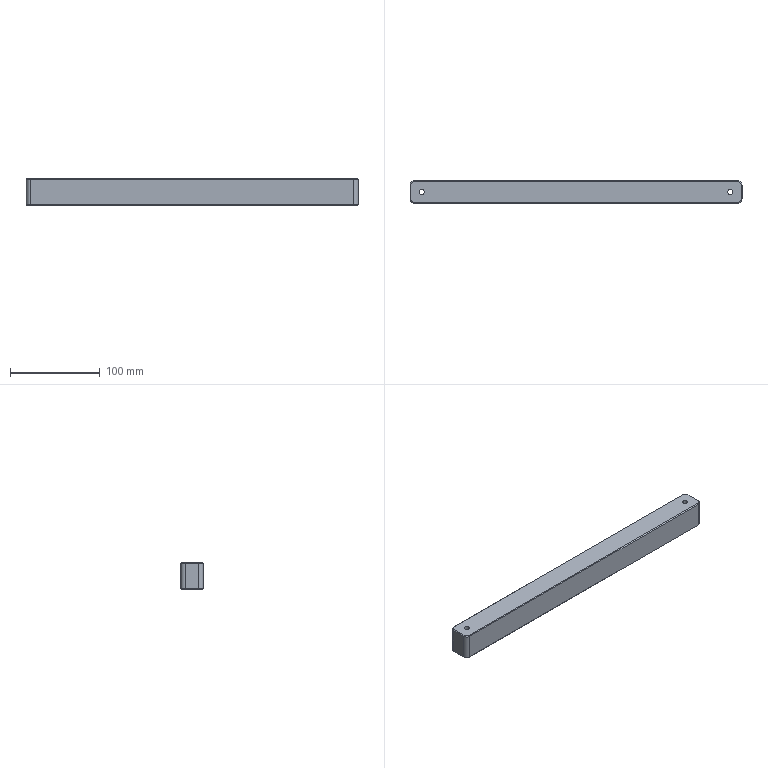Part | SolidWorks | features Chamfer 1, Extrusion 1, Fillet 1, HoleWzd 1 | 1 solid | 36 faces | box 370 x 25 x 30 mm | volume 274027 mm3 | plane 16 | cylinder 12 | cone 8 | commonest cylinder face diameters 10 x8 5.5 x4
STEP:
#1=CARTESIAN_POINT('',(177.,0.,-9.3));
#2=VERTEX_POINT('',#1);
#3=CARTESIAN_POINT('',(167.,0.,-9.3));
#4=VERTEX_POINT('',#3);
#5=CARTESIAN_POINT('',(172.,0.,-9.3));
#6=DIRECTION('',(0.,0.,-1.));
#7=DIRECTION('',(-1.,0.,0.));
#8=AXIS2_PLACEMENT_3D('',#5,#6,#7);
#9=CIRCLE('',#8,5.);
#10=EDGE_CURVE('',#2,#4,#9,.T.);
#11=ORIENTED_EDGE('',*,*,#10,.F.);
#12=CARTESIAN_POINT('',(177.,0.,-15.));
#13=VERTEX_POINT('',#12);
#14=CARTESIAN_POINT('',(177.,0.,-15.));
#15=DIRECTION('',(0.,0.,-1.));
#16=VECTOR('',#15,1000.);
#17=LINE('',#14,#16);
#18=EDGE_CURVE('',#2,#13,#17,.T.);
#19=ORIENTED_EDGE('',*,*,#18,.T.);
#20=CARTESIAN_POINT('',(167.,0.,-15.));
#21=VERTEX_POINT('',#20);
#22=CARTESIAN_POINT('',(172.,0.,-15.));
#23=DIRECTION('',(0.,0.,-1.));
#24=DIRECTION('',(-1.,0.,0.));
#25=AXIS2_PLACEMENT_3D('',#22,#23,#24);
#26=CIRCLE('',#25,5.);
#27=EDGE_CURVE('',#13,#21,#26,.T.);
#28=ORIENTED_EDGE('',*,*,#27,.T.);
#29=CARTESIAN_POINT('',(167.,0.,-15.));
#30=DIRECTION('',(0.,0.,-1.));
#31=VECTOR('',#30,1000.);
#32=LINE('',#29,#31);
#33=EDGE_CURVE('',#4,#21,#32,.T.);
#34=ORIENTED_EDGE('',*,*,#33,.F.);
#35=EDGE_LOOP('',(#11,#19,#28,#34));
#36=FACE_OUTER_BOUND('',#35,.T.);
#37=CARTESIAN_POINT('',(172.,0.,-15.));
#38=DIRECTION('',(0.,0.,-1.));
#39=DIRECTION('',(-1.,0.,0.));
#40=AXIS2_PLACEMENT_3D('',#37,#38,#39);
#41=CYLINDRICAL_SURFACE('',#40,5.);
#42=ADVANCED_FACE('',(#36),#41,.F.);
#43=CARTESIAN_POINT('',(174.75,0.,15.));
#44=VERTEX_POINT('',#43);
#45=CARTESIAN_POINT('',(169.25,0.,15.));
#46=VERTEX_POINT('',#45);
#47=CARTESIAN_POINT('',(172.,0.,15.));
#48=DIRECTION('',(0.,0.,-1.));
#49=DIRECTION('',(-1.,0.,0.));
#50=AXIS2_PLACEMENT_3D('',#47,#48,#49);
#51=CIRCLE('',#50,2.75);
#52=EDGE_CURVE('',#44,#46,#51,.T.);
#53=ORIENTED_EDGE('',*,*,#52,.F.);
#54=CARTESIAN_POINT('',(174.75,0.,-9.3));
#55=VERTEX_POINT('',#54);
#56=CARTESIAN_POINT('',(174.75,0.,-15.));
#57=DIRECTION('',(0.,0.,-1.));
#58=VECTOR('',#57,1000.);
#59=LINE('',#56,#58);
#60=EDGE_CURVE('',#44,#55,#59,.T.);
#61=ORIENTED_EDGE('',*,*,#60,.T.);
#62=CARTESIAN_POINT('',(169.25,0.,-9.3));
#63=VERTEX_POINT('',#62);
#64=CARTESIAN_POINT('',(172.,0.,-9.3));
#65=DIRECTION('',(0.,0.,-1.));
#66=DIRECTION('',(-1.,0.,0.));
#67=AXIS2_PLACEMENT_3D('',#64,#65,#66);
#68=CIRCLE('',#67,2.75);
#69=EDGE_CURVE('',#55,#63,#68,.T.);
#70=ORIENTED_EDGE('',*,*,#69,.T.);
#71=CARTESIAN_POINT('',(169.25,0.,-15.));
#72=DIRECTION('',(0.,0.,-1.));
#73=VECTOR('',#72,1000.);
#74=LINE('',#71,#73);
#75=EDGE_CURVE('',#46,#63,#74,.T.);
#76=ORIENTED_EDGE('',*,*,#75,.F.);
#77=EDGE_LOOP('',(#53,#61,#70,#76));
#78=FACE_OUTER_BOUND('',#77,.T.);
#79=CARTESIAN_POINT('',(172.,0.,-15.));
#80=DIRECTION('',(0.,0.,-1.));
#81=DIRECTION('',(-1.,0.,0.));
#82=AXIS2_PLACEMENT_3D('',#79,#80,#81);
#83=CYLINDRICAL_SURFACE('',#82,2.75);
#84=ADVANCED_FACE('',(#78),#83,.F.);
#85=CARTESIAN_POINT('',(-167.,0.,-9.3));
#86=VERTEX_POINT('',#85);
#87=CARTESIAN_POINT('',(-177.,0.,-9.3));
#88=VERTEX_POINT('',#87);
#89=CARTESIAN_POINT('',(-172.,0.,-9.3));
#90=DIRECTION('',(0.,0.,-1.));
#91=DIRECTION('',(-1.,0.,0.));
#92=AXIS2_PLACEMENT_3D('',#89,#90,#91);
#93=CIRCLE('',#92,5.);
#94=EDGE_CURVE('',#86,#88,#93,.T.);
#95=ORIENTED_EDGE('',*,*,#94,.F.);
#96=CARTESIAN_POINT('',(-167.,0.,-15.));
#97=VERTEX_POINT('',#96);
#98=CARTESIAN_POINT('',(-167.,0.,-15.));
#99=DIRECTION('',(0.,0.,-1.));
#100=VECTOR('',#99,1000.);
#101=LINE('',#98,#100);
#102=EDGE_CURVE('',#86,#97,#101,.T.);
#103=ORIENTED_EDGE('',*,*,#102,.T.);
#104=CARTESIAN_POINT('',(-177.,0.,-15.));
#105=VERTEX_POINT('',#104);
#106=CARTESIAN_POINT('',(-172.,0.,-15.));
#107=DIRECTION('',(0.,0.,-1.));
#108=DIRECTION('',(-1.,0.,0.));
#109=AXIS2_PLACEMENT_3D('',#106,#107,#108);
#110=CIRCLE('',#109,5.);
#111=EDGE_CURVE('',#97,#105,#110,.T.);
#112=ORIENTED_EDGE('',*,*,#111,.T.);
#113=CARTESIAN_POINT('',(-177.,0.,-15.));
#114=DIRECTION('',(0.,0.,-1.));
#115=VECTOR('',#114,1000.);
#116=LINE('',#113,#115);
#117=EDGE_CURVE('',#88,#105,#116,.T.);
#118=ORIENTED_EDGE('',*,*,#117,.F.);
#119=EDGE_LOOP('',(#95,#103,#112,#118));
#120=FACE_OUTER_BOUND('',#119,.T.);
#121=CARTESIAN_POINT('',(-172.,0.,-15.));
#122=DIRECTION('',(0.,0.,-1.));
#123=DIRECTION('',(-1.,0.,0.));
#124=AXIS2_PLACEMENT_3D('',#121,#122,#123);
#125=CYLINDRICAL_SURFACE('',#124,5.);
#126=ADVANCED_FACE('',(#120),#125,.F.);
#127=CARTESIAN_POINT('',(-169.25,0.,15.));
#128=VERTEX_POINT('',#127);
#129=CARTESIAN_POINT('',(-174.75,0.,15.));
#130=VERTEX_POINT('',#129);
#131=CARTESIAN_POINT('',(-172.,0.,15.));
#132=DIRECTION('',(0.,0.,-1.));
#133=DIRECTION('',(-1.,0.,0.));
#134=AXIS2_PLACEMENT_3D('',#131,#132,#133);
#135=CIRCLE('',#134,2.75);
#136=EDGE_CURVE('',#128,#130,#135,.T.);
#137=ORIENTED_EDGE('',*,*,#136,.F.);
#138=CARTESIAN_POINT('',(-169.25,0.,-9.3));
#139=VERTEX_POINT('',#138);
#140=CARTESIAN_POINT('',(-169.25,0.,-15.));
#141=DIRECTION('',(0.,0.,-1.));
#142=VECTOR('',#141,1000.);
#143=LINE('',#140,#142);
#144=EDGE_CURVE('',#128,#139,#143,.T.);
#145=ORIENTED_EDGE('',*,*,#144,.T.);
#146=CARTESIAN_POINT('',(-174.75,0.,-9.3));
#147=VERTEX_POINT('',#146);
#148=CARTESIAN_POINT('',(-172.,0.,-9.3));
#149=DIRECTION('',(0.,0.,-1.));
#150=DIRECTION('',(-1.,0.,0.));
#151=AXIS2_PLACEMENT_3D('',#148,#149,#150);
#152=CIRCLE('',#151,2.75);
#153=EDGE_CURVE('',#139,#147,#152,.T.);
#154=ORIENTED_EDGE('',*,*,#153,.T.);
#155=CARTESIAN_POINT('',(-174.75,0.,-15.));
#156=DIRECTION('',(0.,0.,-1.));
#157=VECTOR('',#156,1000.);
#158=LINE('',#155,#157);
#159=EDGE_CURVE('',#130,#147,#158,.T.);
#160=ORIENTED_EDGE('',*,*,#159,.F.);
#161=EDGE_LOOP('',(#137,#145,#154,#160));
#162=FACE_OUTER_BOUND('',#161,.T.);
#163=CARTESIAN_POINT('',(-172.,0.,-15.));
#164=DIRECTION('',(0.,0.,-1.));
#165=DIRECTION('',(-1.,0.,0.));
#166=AXIS2_PLACEMENT_3D('',#163,#164,#165);
#167=CYLINDRICAL_SURFACE('',#166,2.75);
#168=ADVANCED_FACE('',(#162),#167,.F.);
#169=CARTESIAN_POINT('',(185.,7.5,-14.));
#170=VERTEX_POINT('',#169);
#171=CARTESIAN_POINT('',(185.,7.5,14.));
#172=VERTEX_POINT('',#171);
#173=CARTESIAN_POINT('',(185.,7.5,15.));
#174=DIRECTION('',(0.,0.,1.));
#175=VECTOR('',#174,1000.);
#176=LINE('',#173,#175);
#177=EDGE_CURVE('',#170,#172,#176,.T.);
#178=ORIENTED_EDGE('',*,*,#177,.T.);
#179=CARTESIAN_POINT('',(185.,-7.5,14.));
#180=VERTEX_POINT('',#179);
#181=CARTESIAN_POINT('',(185.,-7.5,14.));
#182=DIRECTION('',(0.,-1.,0.));
#183=VECTOR('',#182,1000.);
#184=LINE('',#181,#183);
#185=EDGE_CURVE('',#172,#180,#184,.T.);
#186=ORIENTED_EDGE('',*,*,#185,.T.);
#187=CARTESIAN_POINT('',(185.,-7.5,-14.));
#188=VERTEX_POINT('',#187);
#189=CARTESIAN_POINT('',(185.,-7.5,15.));
#190=DIRECTION('',(0.,0.,-1.));
#191=VECTOR('',#190,1000.);
#192=LINE('',#189,#191);
#193=EDGE_CURVE('',#180,#188,#192,.T.);
#194=ORIENTED_EDGE('',*,*,#193,.T.);
#195=CARTESIAN_POINT('',(185.,12.5,-14.));
#196=DIRECTION('',(0.,1.,0.));
#197=VECTOR('',#196,1000.);
#198=LINE('',#195,#197);
#199=EDGE_CURVE('',#188,#170,#198,.T.);
#200=ORIENTED_EDGE('',*,*,#199,.T.);
#201=EDGE_LOOP('',(#178,#186,#194,#200));
#202=FACE_OUTER_BOUND('',#201,.T.);
#203=CARTESIAN_POINT('',(185.,12.5,15.));
#204=DIRECTION('',(-1.,0.,0.));
#205=DIRECTION('',(0.,0.,1.));
#206=AXIS2_PLACEMENT_3D('',#203,#204,#205);
#207=PLANE('',#206);
#208=ADVANCED_FACE('',(#202),#207,.F.);
#209=CARTESIAN_POINT('',(-180.,12.5,-14.));
#210=VERTEX_POINT('',#209);
#211=CARTESIAN_POINT('',(-180.,12.5,14.));
#212=VERTEX_POINT('',#211);
#213=CARTESIAN_POINT('',(-180.,12.5,15.));
#214=DIRECTION('',(0.,0.,1.));
#215=VECTOR('',#214,1000.);
#216=LINE('',#213,#215);
#217=EDGE_CURVE('',#210,#212,#216,.T.);
#218=ORIENTED_EDGE('',*,*,#217,.T.);
#219=CARTESIAN_POINT('',(180.,12.5,14.));
#220=VERTEX_POINT('',#219);
#221=CARTESIAN_POINT('',(180.,12.5,14.));
#222=DIRECTION('',(1.,0.,0.));
#223=VECTOR('',#222,1000.);
#224=LINE('',#221,#223);
#225=EDGE_CURVE('',#212,#220,#224,.T.);
#226=ORIENTED_EDGE('',*,*,#225,.T.);
#227=CARTESIAN_POINT('',(180.,12.5,-14.));
#228=VERTEX_POINT('',#227);
#229=CARTESIAN_POINT('',(180.,12.5,15.));
#230=DIRECTION('',(0.,0.,-1.));
#231=VECTOR('',#230,1000.);
#232=LINE('',#229,#231);
#233=EDGE_CURVE('',#220,#228,#232,.T.);
#234=ORIENTED_EDGE('',*,*,#233,.T.);
#235=CARTESIAN_POINT('',(-185.,12.5,-14.));
#236=DIRECTION('',(-1.,0.,0.));
#237=VECTOR('',#236,1000.);
#238=LINE('',#235,#237);
#239=EDGE_CURVE('',#228,#210,#238,.T.);
#240=ORIENTED_EDGE('',*,*,#239,.T.);
#241=EDGE_LOOP('',(#218,#226,#234,#240));
#242=FACE_OUTER_BOUND('',#241,.T.);
#243=CARTESIAN_POINT('',(-185.,12.5,15.));
#244=DIRECTION('',(0.,-1.,0.));
#245=DIRECTION('',(0.,0.,-1.));
#246=AXIS2_PLACEMENT_3D('',#243,#244,#245);
#247=PLANE('',#246);
#248=ADVANCED_FACE('',(#242),#247,.F.);
#249=CARTESIAN_POINT('',(-185.,-7.5,-14.));
#250=VERTEX_POINT('',#249);
#251=CARTESIAN_POINT('',(-185.,-7.5,14.));
#252=VERTEX_POINT('',#251);
#253=CARTESIAN_POINT('',(-185.,-7.5,15.));
#254=DIRECTION('',(0.,0.,1.));
#255=VECTOR('',#254,1000.);
#256=LINE('',#253,#255);
#257=EDGE_CURVE('',#250,#252,#256,.T.);
#258=ORIENTED_EDGE('',*,*,#257,.T.);
#259=CARTESIAN_POINT('',(-185.,7.5,14.));
#260=VERTEX_POINT('',#259);
#261=CARTESIAN_POINT('',(-185.,7.5,14.));
#262=DIRECTION('',(0.,1.,0.));
#263=VECTOR('',#262,1000.);
#264=LINE('',#261,#263);
#265=EDGE_CURVE('',#252,#260,#264,.T.);
#266=ORIENTED_EDGE('',*,*,#265,.T.);
#267=CARTESIAN_POINT('',(-185.,7.5,-14.));
#268=VERTEX_POINT('',#267);
#269=CARTESIAN_POINT('',(-185.,7.5,15.));
#270=DIRECTION('',(0.,0.,-1.));
#271=VECTOR('',#270,1000.);
#272=LINE('',#269,#271);
#273=EDGE_CURVE('',#260,#268,#272,.T.);
#274=ORIENTED_EDGE('',*,*,#273,.T.);
#275=CARTESIAN_POINT('',(-185.,12.5,-14.));
#276=DIRECTION('',(0.,-1.,0.));
#277=VECTOR('',#276,1000.);
#278=LINE('',#275,#277);
#279=EDGE_CURVE('',#268,#250,#278,.T.);
#280=ORIENTED_EDGE('',*,*,#279,.T.);
#281=EDGE_LOOP('',(#258,#266,#274,#280));
#282=FACE_OUTER_BOUND('',#281,.T.);
#283=CARTESIAN_POINT('',(-185.,12.5,15.));
#284=DIRECTION('',(1.,0.,0.));
#285=DIRECTION('',(0.,0.,-1.));
#286=AXIS2_PLACEMENT_3D('',#283,#284,#285);
#287=PLANE('',#286);
#288=ADVANCED_FACE('',(#282),#287,.F.);
#289=CARTESIAN_POINT('',(180.,-12.5,-14.));
#290=VERTEX_POINT('',#289);
#291=CARTESIAN_POINT('',(180.,-12.5,14.));
#292=VERTEX_POINT('',#291);
#293=CARTESIAN_POINT('',(180.,-12.5,15.));
#294=DIRECTION('',(0.,0.,1.));
#295=VECTOR('',#294,1000.);
#296=LINE('',#293,#295);
#297=EDGE_CURVE('',#290,#292,#296,.T.);
#298=ORIENTED_EDGE('',*,*,#297,.T.);
#299=CARTESIAN_POINT('',(-180.,-12.5,14.));
#300=VERTEX_POINT('',#299);
#301=CARTESIAN_POINT('',(-180.,-12.5,14.));
#302=DIRECTION('',(-1.,0.,0.));
#303=VECTOR('',#302,1000.);
#304=LINE('',#301,#303);
#305=EDGE_CURVE('',#292,#300,#304,.T.);
#306=ORIENTED_EDGE('',*,*,#305,.T.);
#307=CARTESIAN_POINT('',(-180.,-12.5,-14.));
#308=VERTEX_POINT('',#307);
#309=CARTESIAN_POINT('',(-180.,-12.5,15.));
#310=DIRECTION('',(0.,0.,-1.));
#311=VECTOR('',#310,1000.);
#312=LINE('',#309,#311);
#313=EDGE_CURVE('',#300,#308,#312,.T.);
#314=ORIENTED_EDGE('',*,*,#313,.T.);
#315=CARTESIAN_POINT('',(-185.,-12.5,-14.));
#316=DIRECTION('',(1.,0.,0.));
#317=VECTOR('',#316,1000.);
#318=LINE('',#315,#317);
#319=EDGE_CURVE('',#308,#290,#318,.T.);
#320=ORIENTED_EDGE('',*,*,#319,.T.);
#321=EDGE_LOOP('',(#298,#306,#314,#320));
#322=FACE_OUTER_BOUND('',#321,.T.);
#323=CARTESIAN_POINT('',(-185.,-12.5,15.));
#324=DIRECTION('',(0.,1.,0.));
#325=DIRECTION('',(0.,0.,1.));
#326=AXIS2_PLACEMENT_3D('',#323,#324,#325);
#327=PLANE('',#326);
#328=ADVANCED_FACE('',(#322),#327,.F.);
#329=CARTESIAN_POINT('',(172.,0.,15.));
#330=DIRECTION('',(0.,0.,-1.));
#331=DIRECTION('',(-1.,0.,0.));
#332=AXIS2_PLACEMENT_3D('',#329,#330,#331);
#333=CIRCLE('',#332,2.75);
#334=EDGE_CURVE('',#46,#44,#333,.T.);
#335=ORIENTED_EDGE('',*,*,#334,.T.);
#336=ORIENTED_EDGE('',*,*,#52,.T.);
#337=EDGE_LOOP('',(#335,#336));
#338=FACE_BOUND('',#337,.T.);
#339=CARTESIAN_POINT('',(-172.,0.,15.));
#340=DIRECTION('',(0.,0.,-1.));
#341=DIRECTION('',(-1.,0.,0.));
#342=AXIS2_PLACEMENT_3D('',#339,#340,#341);
#343=CIRCLE('',#342,2.75);
#344=EDGE_CURVE('',#130,#128,#343,.T.);
#345=ORIENTED_EDGE('',*,*,#344,.T.);
#346=ORIENTED_EDGE('',*,*,#136,.T.);
#347=EDGE_LOOP('',(#345,#346));
#348=FACE_BOUND('',#347,.T.);
#349=CARTESIAN_POINT('',(184.,-7.5,15.));
#350=VERTEX_POINT('',#349);
#351=CARTESIAN_POINT('',(184.,7.5,15.));
#352=VERTEX_POINT('',#351);
#353=CARTESIAN_POINT('',(184.,7.5,15.));
#354=DIRECTION('',(0.,1.,0.));
#355=VECTOR('',#354,1000.);
#356=LINE('',#353,#355);
#357=EDGE_CURVE('',#350,#352,#356,.T.);
#358=ORIENTED_EDGE('',*,*,#357,.T.);
#359=CARTESIAN_POINT('',(180.,11.5,15.));
#360=VERTEX_POINT('',#359);
#361=CARTESIAN_POINT('',(180.,7.5,15.));
#362=DIRECTION('',(0.,0.,1.));
#363=DIRECTION('',(1.,0.,0.));
#364=AXIS2_PLACEMENT_3D('',#361,#362,#363);
#365=CIRCLE('',#364,4.);
#366=EDGE_CURVE('',#352,#360,#365,.T.);
#367=ORIENTED_EDGE('',*,*,#366,.T.);
#368=CARTESIAN_POINT('',(-180.,11.5,15.));
#369=VERTEX_POINT('',#368);
#370=CARTESIAN_POINT('',(-180.,11.5,15.));
#371=DIRECTION('',(-1.,0.,0.));
#372=VECTOR('',#371,1000.);
#373=LINE('',#370,#372);
#374=EDGE_CURVE('',#360,#369,#373,.T.);
#375=ORIENTED_EDGE('',*,*,#374,.T.);
#376=CARTESIAN_POINT('',(-184.,7.5,15.));
#377=VERTEX_POINT('',#376);
#378=CARTESIAN_POINT('',(-180.,7.5,15.));
#379=DIRECTION('',(0.,0.,1.));
#380=DIRECTION('',(1.,0.,0.));
#381=AXIS2_PLACEMENT_3D('',#378,#379,#380);
#382=CIRCLE('',#381,4.);
#383=EDGE_CURVE('',#369,#377,#382,.T.);
#384=ORIENTED_EDGE('',*,*,#383,.T.);
#385=CARTESIAN_POINT('',(-184.,-7.5,15.));
#386=VERTEX_POINT('',#385);
#387=CARTESIAN_POINT('',(-184.,-7.5,15.));
#388=DIRECTION('',(0.,-1.,0.));
#389=VECTOR('',#388,1000.);
#390=LINE('',#387,#389);
#391=EDGE_CURVE('',#377,#386,#390,.T.);
#392=ORIENTED_EDGE('',*,*,#391,.T.);
#393=CARTESIAN_POINT('',(-180.,-11.5,15.));
#394=VERTEX_POINT('',#393);
#395=CARTESIAN_POINT('',(-180.,-7.5,15.));
#396=DIRECTION('',(0.,0.,1.));
#397=DIRECTION('',(1.,0.,0.));
#398=AXIS2_PLACEMENT_3D('',#395,#396,#397);
#399=CIRCLE('',#398,4.);
#400=EDGE_CURVE('',#386,#394,#399,.T.);
#401=ORIENTED_EDGE('',*,*,#400,.T.);
#402=CARTESIAN_POINT('',(180.,-11.5,15.));
#403=VERTEX_POINT('',#402);
#404=CARTESIAN_POINT('',(180.,-11.5,15.));
#405=DIRECTION('',(1.,0.,0.));
#406=VECTOR('',#405,1000.);
#407=LINE('',#404,#406);
#408=EDGE_CURVE('',#394,#403,#407,.T.);
#409=ORIENTED_EDGE('',*,*,#408,.T.);
#410=CARTESIAN_POINT('',(180.,-7.5,15.));
#411=DIRECTION('',(0.,0.,1.));
#412=DIRECTION('',(1.,0.,0.));
#413=AXIS2_PLACEMENT_3D('',#410,#411,#412);
#414=CIRCLE('',#413,4.);
#415=EDGE_CURVE('',#403,#350,#414,.T.);
#416=ORIENTED_EDGE('',*,*,#415,.T.);
#417=EDGE_LOOP('',(#358,#367,#375,#384,#392,#401,#409,#416));
#418=FACE_OUTER_BOUND('',#417,.T.);
#419=CARTESIAN_POINT('',(185.,-12.5,15.));
#420=DIRECTION('',(0.,0.,1.));
#421=DIRECTION('',(1.,0.,0.));
#422=AXIS2_PLACEMENT_3D('',#419,#420,#421);
#423=PLANE('',#422);
#424=ADVANCED_FACE('',(#338,#348,#418),#423,.T.);
#425=CARTESIAN_POINT('',(172.,0.,-15.));
#426=DIRECTION('',(0.,0.,-1.));
#427=DIRECTION('',(-1.,0.,0.));
#428=AXIS2_PLACEMENT_3D('',#425,#426,#427);
#429=CIRCLE('',#428,5.);
#430=EDGE_CURVE('',#21,#13,#429,.T.);
#431=ORIENTED_EDGE('',*,*,#430,.F.);
#432=ORIENTED_EDGE('',*,*,#27,.F.);
#433=EDGE_LOOP('',(#431,#432));
#434=FACE_BOUND('',#433,.T.);
#435=CARTESIAN_POINT('',(-172.,0.,-15.));
#436=DIRECTION('',(0.,0.,-1.));
#437=DIRECTION('',(-1.,0.,0.));
#438=AXIS2_PLACEMENT_3D('',#435,#436,#437);
#439=CIRCLE('',#438,5.);
#440=EDGE_CURVE('',#105,#97,#439,.T.);
#441=ORIENTED_EDGE('',*,*,#440,.F.);
#442=ORIENTED_EDGE('',*,*,#111,.F.);
#443=EDGE_LOOP('',(#441,#442));
#444=FACE_BOUND('',#443,.T.);
#445=CARTESIAN_POINT('',(-184.,7.5,-15.));
#446=VERTEX_POINT('',#445);
#447=CARTESIAN_POINT('',(-180.,11.5,-15.));
#448=VERTEX_POINT('',#447);
#449=CARTESIAN_POINT('',(-180.,7.5,-15.));
#450=DIRECTION('',(0.,0.,-1.));
#451=DIRECTION('',(1.,0.,0.));
#452=AXIS2_PLACEMENT_3D('',#449,#450,#451);
#453=CIRCLE('',#452,4.);
#454=EDGE_CURVE('',#446,#448,#453,.T.);
#455=ORIENTED_EDGE('',*,*,#454,.T.);
#456=CARTESIAN_POINT('',(180.,11.5,-15.));
#457=VERTEX_POINT('',#456);
#458=CARTESIAN_POINT('',(185.,11.5,-15.));
#459=DIRECTION('',(1.,0.,0.));
#460=VECTOR('',#459,1000.);
#461=LINE('',#458,#460);
#462=EDGE_CURVE('',#448,#457,#461,.T.);
#463=ORIENTED_EDGE('',*,*,#462,.T.);
#464=CARTESIAN_POINT('',(184.,7.5,-15.));
#465=VERTEX_POINT('',#464);
#466=CARTESIAN_POINT('',(180.,7.5,-15.));
#467=DIRECTION('',(0.,0.,-1.));
#468=DIRECTION('',(1.,0.,0.));
#469=AXIS2_PLACEMENT_3D('',#466,#467,#468);
#470=CIRCLE('',#469,4.);
#471=EDGE_CURVE('',#457,#465,#470,.T.);
#472=ORIENTED_EDGE('',*,*,#471,.T.);
#473=CARTESIAN_POINT('',(184.,-7.5,-15.));
#474=VERTEX_POINT('',#473);
#475=CARTESIAN_POINT('',(184.,-12.5,-15.));
#476=DIRECTION('',(0.,-1.,0.));
#477=VECTOR('',#476,1000.);
#478=LINE('',#475,#477);
#479=EDGE_CURVE('',#465,#474,#478,.T.);
#480=ORIENTED_EDGE('',*,*,#479,.T.);
#481=CARTESIAN_POINT('',(180.,-11.5,-15.));
#482=VERTEX_POINT('',#481);
#483=CARTESIAN_POINT('',(180.,-7.5,-15.));
#484=DIRECTION('',(0.,0.,-1.));
#485=DIRECTION('',(1.,0.,0.));
#486=AXIS2_PLACEMENT_3D('',#483,#484,#485);
#487=CIRCLE('',#486,4.);
#488=EDGE_CURVE('',#474,#482,#487,.T.);
#489=ORIENTED_EDGE('',*,*,#488,.T.);
#490=CARTESIAN_POINT('',(-180.,-11.5,-15.));
#491=VERTEX_POINT('',#490);
#492=CARTESIAN_POINT('',(185.,-11.5,-15.));
#493=DIRECTION('',(-1.,0.,0.));
#494=VECTOR('',#493,1000.);
#495=LINE('',#492,#494);
#496=EDGE_CURVE('',#482,#491,#495,.T.);
#497=ORIENTED_EDGE('',*,*,#496,.T.);
#498=CARTESIAN_POINT('',(-184.,-7.5,-15.));
#499=VERTEX_POINT('',#498);
#500=CARTESIAN_POINT('',(-180.,-7.5,-15.));
#501=DIRECTION('',(0.,0.,-1.));
#502=DIRECTION('',(1.,0.,0.));
#503=AXIS2_PLACEMENT_3D('',#500,#501,#502);
#504=CIRCLE('',#503,4.);
#505=EDGE_CURVE('',#491,#499,#504,.T.);
#506=ORIENTED_EDGE('',*,*,#505,.T.);
#507=CARTESIAN_POINT('',(-184.,-12.5,-15.));
#508=DIRECTION('',(0.,1.,0.));
#509=VECTOR('',#508,1000.);
#510=LINE('',#507,#509);
#511=EDGE_CURVE('',#499,#446,#510,.T.);
#512=ORIENTED_EDGE('',*,*,#511,.T.);
#513=EDGE_LOOP('',(#455,#463,#472,#480,#489,#497,#506,#512));
#514=FACE_OUTER_BOUND('',#513,.T.);
#515=CARTESIAN_POINT('',(185.,-12.5,-15.));
#516=DIRECTION('',(0.,0.,1.));
#517=DIRECTION('',(1.,0.,0.));
#518=AXIS2_PLACEMENT_3D('',#515,#516,#517);
#519=PLANE('',#518);
#520=ADVANCED_FACE('',(#434,#444,#514),#519,.F.);
#521=ORIENTED_EDGE('',*,*,#273,.F.);
#522=CARTESIAN_POINT('',(-180.,7.5,14.));
#523=DIRECTION('',(0.,0.,-1.));
#524=DIRECTION('',(1.,0.,0.));
#525=AXIS2_PLACEMENT_3D('',#522,#523,#524);
#526=CIRCLE('',#525,5.);
#527=EDGE_CURVE('',#260,#212,#526,.T.);
#528=ORIENTED_EDGE('',*,*,#527,.T.);
#529=ORIENTED_EDGE('',*,*,#217,.F.);
#530=CARTESIAN_POINT('',(-180.,7.5,-14.));
#531=DIRECTION('',(0.,0.,1.));
#532=DIRECTION('',(1.,0.,0.));
#533=AXIS2_PLACEMENT_3D('',#530,#531,#532);
#534=CIRCLE('',#533,5.);
#535=EDGE_CURVE('',#210,#268,#534,.T.);
#536=ORIENTED_EDGE('',*,*,#535,.T.);
#537=EDGE_LOOP('',(#521,#528,#529,#536));
#538=FACE_OUTER_BOUND('',#537,.T.);
#539=CARTESIAN_POINT('',(-180.,7.5,15.));
#540=DIRECTION('',(0.,0.,-1.));
#541=DIRECTION('',(-1.,0.,0.));
#542=AXIS2_PLACEMENT_3D('',#539,#540,#541);
#543=CYLINDRICAL_SURFACE('',#542,5.);
#544=ADVANCED_FACE('',(#538),#543,.T.);
#545=ORIENTED_EDGE('',*,*,#313,.F.);
#546=CARTESIAN_POINT('',(-180.,-7.5,14.));
#547=DIRECTION('',(0.,0.,-1.));
#548=DIRECTION('',(1.,0.,0.));
#549=AXIS2_PLACEMENT_3D('',#546,#547,#548);
#550=CIRCLE('',#549,5.);
#551=EDGE_CURVE('',#300,#252,#550,.T.);
#552=ORIENTED_EDGE('',*,*,#551,.T.);
#553=ORIENTED_EDGE('',*,*,#257,.F.);
#554=CARTESIAN_POINT('',(-180.,-7.5,-14.));
#555=DIRECTION('',(0.,0.,1.));
#556=DIRECTION('',(1.,0.,0.));
#557=AXIS2_PLACEMENT_3D('',#554,#555,#556);
#558=CIRCLE('',#557,5.);
#559=EDGE_CURVE('',#250,#308,#558,.T.);
#560=ORIENTED_EDGE('',*,*,#559,.T.);
#561=EDGE_LOOP('',(#545,#552,#553,#560));
#562=FACE_OUTER_BOUND('',#561,.T.);
#563=CARTESIAN_POINT('',(-180.,-7.5,15.));
#564=DIRECTION('',(0.,0.,-1.));
#565=DIRECTION('',(-1.,0.,0.));
#566=AXIS2_PLACEMENT_3D('',#563,#564,#565);
#567=CYLINDRICAL_SURFACE('',#566,5.);
#568=ADVANCED_FACE('',(#562),#567,.T.);
#569=ORIENTED_EDGE('',*,*,#193,.F.);
#570=CARTESIAN_POINT('',(180.,-7.5,14.));
#571=DIRECTION('',(0.,0.,-1.));
#572=DIRECTION('',(1.,0.,0.));
#573=AXIS2_PLACEMENT_3D('',#570,#571,#572);
#574=CIRCLE('',#573,5.);
#575=EDGE_CURVE('',#180,#292,#574,.T.);
#576=ORIENTED_EDGE('',*,*,#575,.T.);
#577=ORIENTED_EDGE('',*,*,#297,.F.);
#578=CARTESIAN_POINT('',(180.,-7.5,-14.));
#579=DIRECTION('',(0.,0.,1.));
#580=DIRECTION('',(1.,0.,0.));
#581=AXIS2_PLACEMENT_3D('',#578,#579,#580);
#582=CIRCLE('',#581,5.);
#583=EDGE_CURVE('',#290,#188,#582,.T.);
#584=ORIENTED_EDGE('',*,*,#583,.T.);
#585=EDGE_LOOP('',(#569,#576,#577,#584));
#586=FACE_OUTER_BOUND('',#585,.T.);
#587=CARTESIAN_POINT('',(180.,-7.5,15.));
#588=DIRECTION('',(0.,0.,-1.));
#589=DIRECTION('',(-1.,0.,0.));
#590=AXIS2_PLACEMENT_3D('',#587,#588,#589);
#591=CYLINDRICAL_SURFACE('',#590,5.);
#592=ADVANCED_FACE('',(#586),#591,.T.);
#593=ORIENTED_EDGE('',*,*,#233,.F.);
#594=CARTESIAN_POINT('',(180.,7.5,14.));
#595=DIRECTION('',(0.,0.,-1.));
#596=DIRECTION('',(1.,0.,0.));
#597=AXIS2_PLACEMENT_3D('',#594,#595,#596);
#598=CIRCLE('',#597,5.);
#599=EDGE_CURVE('',#220,#172,#598,.T.);
#600=ORIENTED_EDGE('',*,*,#599,.T.);
#601=ORIENTED_EDGE('',*,*,#177,.F.);
#602=CARTESIAN_POINT('',(180.,7.5,-14.));
#603=DIRECTION('',(0.,0.,1.));
#604=DIRECTION('',(1.,0.,0.));
#605=AXIS2_PLACEMENT_3D('',#602,#603,#604);
#606=CIRCLE('',#605,5.);
#607=EDGE_CURVE('',#170,#228,#606,.T.);
#608=ORIENTED_EDGE('',*,*,#607,.T.);
#609=EDGE_LOOP('',(#593,#600,#601,#608));
#610=FACE_OUTER_BOUND('',#609,.T.);
#611=CARTESIAN_POINT('',(180.,7.5,15.));
#612=DIRECTION('',(0.,0.,-1.));
#613=DIRECTION('',(-1.,0.,0.));
#614=AXIS2_PLACEMENT_3D('',#611,#612,#613);
#615=CYLINDRICAL_SURFACE('',#614,5.);
#616=ADVANCED_FACE('',(#610),#615,.T.);
#617=CARTESIAN_POINT('',(-185.,-7.5,14.));
#618=DIRECTION('',(0.7071,0.,0.7071));
#619=VECTOR('',#618,1000.);
#620=LINE('',#617,#619);
#621=EDGE_CURVE('',#252,#386,#620,.T.);
#622=ORIENTED_EDGE('',*,*,#621,.F.);
#623=ORIENTED_EDGE('',*,*,#551,.F.);
#624=CARTESIAN_POINT('',(-180.,-11.5,15.));
#625=DIRECTION('',(0.,-0.7071,-0.7071));
#626=VECTOR('',#625,1000.);
#627=LINE('',#624,#626);
#628=EDGE_CURVE('',#394,#300,#627,.T.);
#629=ORIENTED_EDGE('',*,*,#628,.F.);
#630=ORIENTED_EDGE('',*,*,#400,.F.);
#631=EDGE_LOOP('',(#622,#623,#629,#630));
#632=FACE_OUTER_BOUND('',#631,.T.);
#633=CARTESIAN_POINT('',(-180.,-7.5,15.));
#634=DIRECTION('',(0.,0.,-1.));
#635=DIRECTION('',(-1.,0.,0.));
#636=AXIS2_PLACEMENT_3D('',#633,#634,#635);
#637=CONICAL_SURFACE('',#636,4.,0.7854);
#638=ADVANCED_FACE('',(#632),#637,.T.);
#639=ORIENTED_EDGE('',*,*,#628,.T.);
#640=ORIENTED_EDGE('',*,*,#305,.F.);
#641=CARTESIAN_POINT('',(180.,-11.5,15.));
#642=DIRECTION('',(0.,-0.7071,-0.7071));
#643=VECTOR('',#642,1000.);
#644=LINE('',#641,#643);
#645=EDGE_CURVE('',#403,#292,#644,.T.);
#646=ORIENTED_EDGE('',*,*,#645,.F.);
#647=ORIENTED_EDGE('',*,*,#408,.F.);
#648=EDGE_LOOP('',(#639,#640,#646,#647));
#649=FACE_OUTER_BOUND('',#648,.T.);
#650=CARTESIAN_POINT('',(185.,-11.5,15.));
#651=DIRECTION('',(0.,-0.7071,0.7071));
#652=DIRECTION('',(0.,-0.7071,-0.7071));
#653=AXIS2_PLACEMENT_3D('',#650,#651,#652);
#654=PLANE('',#653);
#655=ADVANCED_FACE('',(#649),#654,.T.);
#656=ORIENTED_EDGE('',*,*,#621,.T.);
#657=ORIENTED_EDGE('',*,*,#391,.F.);
#658=CARTESIAN_POINT('',(-185.,7.5,14.));
#659=DIRECTION('',(0.7071,0.,0.7071));
#660=VECTOR('',#659,1000.);
#661=LINE('',#658,#660);
#662=EDGE_CURVE('',#260,#377,#661,.T.);
#663=ORIENTED_EDGE('',*,*,#662,.F.);
#664=ORIENTED_EDGE('',*,*,#265,.F.);
#665=EDGE_LOOP('',(#656,#657,#663,#664));
#666=FACE_OUTER_BOUND('',#665,.T.);
#667=CARTESIAN_POINT('',(-184.,-12.5,15.));
#668=DIRECTION('',(-0.7071,0.,0.7071));
#669=DIRECTION('',(0.7071,0.,0.7071));
#670=AXIS2_PLACEMENT_3D('',#667,#668,#669);
#671=PLANE('',#670);
#672=ADVANCED_FACE('',(#666),#671,.T.);
#673=ORIENTED_EDGE('',*,*,#645,.T.);
#674=ORIENTED_EDGE('',*,*,#575,.F.);
#675=CARTESIAN_POINT('',(184.,-7.5,15.));
#676=DIRECTION('',(0.7071,0.,-0.7071));
#677=VECTOR('',#676,1000.);
#678=LINE('',#675,#677);
#679=EDGE_CURVE('',#350,#180,#678,.T.);
#680=ORIENTED_EDGE('',*,*,#679,.F.);
#681=ORIENTED_EDGE('',*,*,#415,.F.);
#682=EDGE_LOOP('',(#673,#674,#680,#681));
#683=FACE_OUTER_BOUND('',#682,.T.);
#684=CARTESIAN_POINT('',(180.,-7.5,15.));
#685=DIRECTION('',(0.,0.,-1.));
#686=DIRECTION('',(-1.,0.,0.));
#687=AXIS2_PLACEMENT_3D('',#684,#685,#686);
#688=CONICAL_SURFACE('',#687,4.,0.7854);
#689=ADVANCED_FACE('',(#683),#688,.T.);
#690=ORIENTED_EDGE('',*,*,#662,.T.);
#691=ORIENTED_EDGE('',*,*,#383,.F.);
#692=CARTESIAN_POINT('',(-180.,12.5,14.));
#693=DIRECTION('',(0.,-0.7071,0.7071));
#694=VECTOR('',#693,1000.);
#695=LINE('',#692,#694);
#696=EDGE_CURVE('',#212,#369,#695,.T.);
#697=ORIENTED_EDGE('',*,*,#696,.F.);
#698=ORIENTED_EDGE('',*,*,#527,.F.);
#699=EDGE_LOOP('',(#690,#691,#697,#698));
#700=FACE_OUTER_BOUND('',#699,.T.);
#701=CARTESIAN_POINT('',(-180.,7.5,15.));
#702=DIRECTION('',(0.,0.,-1.));
#703=DIRECTION('',(-1.,0.,0.));
#704=AXIS2_PLACEMENT_3D('',#701,#702,#703);
#705=CONICAL_SURFACE('',#704,4.,0.7854);
#706=ADVANCED_FACE('',(#700),#705,.T.);
#707=ORIENTED_EDGE('',*,*,#679,.T.);
#708=ORIENTED_EDGE('',*,*,#185,.F.);
#709=CARTESIAN_POINT('',(184.,7.5,15.));
#710=DIRECTION('',(0.7071,0.,-0.7071));
#711=VECTOR('',#710,1000.);
#712=LINE('',#709,#711);
#713=EDGE_CURVE('',#352,#172,#712,.T.);
#714=ORIENTED_EDGE('',*,*,#713,.F.);
#715=ORIENTED_EDGE('',*,*,#357,.F.);
#716=EDGE_LOOP('',(#707,#708,#714,#715));
#717=FACE_OUTER_BOUND('',#716,.T.);
#718=CARTESIAN_POINT('',(184.,-12.5,15.));
#719=DIRECTION('',(0.7071,0.,0.7071));
#720=DIRECTION('',(0.7071,0.,-0.7071));
#721=AXIS2_PLACEMENT_3D('',#718,#719,#720);
#722=PLANE('',#721);
#723=ADVANCED_FACE('',(#717),#722,.T.);
#724=ORIENTED_EDGE('',*,*,#696,.T.);
#725=ORIENTED_EDGE('',*,*,#374,.F.);
#726=CARTESIAN_POINT('',(180.,12.5,14.));
#727=DIRECTION('',(0.,-0.7071,0.7071));
#728=VECTOR('',#727,1000.);
#729=LINE('',#726,#728);
#730=EDGE_CURVE('',#220,#360,#729,.T.);
#731=ORIENTED_EDGE('',*,*,#730,.F.);
#732=ORIENTED_EDGE('',*,*,#225,.F.);
#733=EDGE_LOOP('',(#724,#725,#731,#732));
#734=FACE_OUTER_BOUND('',#733,.T.);
#735=CARTESIAN_POINT('',(185.,11.5,15.));
#736=DIRECTION('',(0.,0.7071,0.7071));
#737=DIRECTION('',(0.,-0.7071,0.7071));
#738=AXIS2_PLACEMENT_3D('',#735,#736,#737);
#739=PLANE('',#738);
#740=ADVANCED_FACE('',(#734),#739,.T.);
#741=ORIENTED_EDGE('',*,*,#713,.T.);
#742=ORIENTED_EDGE('',*,*,#599,.F.);
#743=ORIENTED_EDGE('',*,*,#730,.T.);
#744=ORIENTED_EDGE('',*,*,#366,.F.);
#745=EDGE_LOOP('',(#741,#742,#743,#744));
#746=FACE_OUTER_BOUND('',#745,.T.);
#747=CARTESIAN_POINT('',(180.,7.5,15.));
#748=DIRECTION('',(0.,0.,-1.));
#749=DIRECTION('',(-1.,0.,0.));
#750=AXIS2_PLACEMENT_3D('',#747,#748,#749);
#751=CONICAL_SURFACE('',#750,4.,0.7854);
#752=ADVANCED_FACE('',(#746),#751,.T.);
#753=CARTESIAN_POINT('',(-180.,-11.5,-15.));
#754=DIRECTION('',(0.,-0.7071,0.7071));
#755=VECTOR('',#754,1000.);
#756=LINE('',#753,#755);
#757=EDGE_CURVE('',#491,#308,#756,.T.);
#758=ORIENTED_EDGE('',*,*,#757,.F.);
#759=ORIENTED_EDGE('',*,*,#496,.F.);
#760=CARTESIAN_POINT('',(180.,-12.5,-14.));
#761=DIRECTION('',(0.,0.7071,-0.7071));
#762=VECTOR('',#761,1000.);
#763=LINE('',#760,#762);
#764=EDGE_CURVE('',#290,#482,#763,.T.);
#765=ORIENTED_EDGE('',*,*,#764,.F.);
#766=ORIENTED_EDGE('',*,*,#319,.F.);
#767=EDGE_LOOP('',(#758,#759,#765,#766));
#768=FACE_OUTER_BOUND('',#767,.T.);
#769=CARTESIAN_POINT('',(-185.,-12.5,-14.));
#770=DIRECTION('',(0.,0.7071,0.7071));
#771=DIRECTION('',(0.,-0.7071,0.7071));
#772=AXIS2_PLACEMENT_3D('',#769,#770,#771);
#773=PLANE('',#772);
#774=ADVANCED_FACE('',(#768),#773,.F.);
#775=ORIENTED_EDGE('',*,*,#764,.T.);
#776=ORIENTED_EDGE('',*,*,#488,.F.);
#777=CARTESIAN_POINT('',(185.,-7.5,-14.));
#778=DIRECTION('',(-0.7071,0.,-0.7071));
#779=VECTOR('',#778,1000.);
#780=LINE('',#777,#779);
#781=EDGE_CURVE('',#188,#474,#780,.T.);
#782=ORIENTED_EDGE('',*,*,#781,.F.);
#783=ORIENTED_EDGE('',*,*,#583,.F.);
#784=EDGE_LOOP('',(#775,#776,#782,#783));
#785=FACE_OUTER_BOUND('',#784,.T.);
#786=CARTESIAN_POINT('',(180.,-7.5,-15.));
#787=DIRECTION('',(0.,0.,1.));
#788=DIRECTION('',(1.,0.,0.));
#789=AXIS2_PLACEMENT_3D('',#786,#787,#788);
#790=CONICAL_SURFACE('',#789,4.,0.7854);
#791=ADVANCED_FACE('',(#785),#790,.T.);
#792=ORIENTED_EDGE('',*,*,#757,.T.);
#793=ORIENTED_EDGE('',*,*,#559,.F.);
#794=CARTESIAN_POINT('',(-184.,-7.5,-15.));
#795=DIRECTION('',(-0.7071,0.,0.7071));
#796=VECTOR('',#795,1000.);
#797=LINE('',#794,#796);
#798=EDGE_CURVE('',#499,#250,#797,.T.);
#799=ORIENTED_EDGE('',*,*,#798,.F.);
#800=ORIENTED_EDGE('',*,*,#505,.F.);
#801=EDGE_LOOP('',(#792,#793,#799,#800));
#802=FACE_OUTER_BOUND('',#801,.T.);
#803=CARTESIAN_POINT('',(-180.,-7.5,-15.));
#804=DIRECTION('',(0.,0.,1.));
#805=DIRECTION('',(1.,0.,0.));
#806=AXIS2_PLACEMENT_3D('',#803,#804,#805);
#807=CONICAL_SURFACE('',#806,4.,0.7854);
#808=ADVANCED_FACE('',(#802),#807,.T.);
#809=ORIENTED_EDGE('',*,*,#781,.T.);
#810=ORIENTED_EDGE('',*,*,#479,.F.);
#811=CARTESIAN_POINT('',(185.,7.5,-14.));
#812=DIRECTION('',(-0.7071,0.,-0.7071));
#813=VECTOR('',#812,1000.);
#814=LINE('',#811,#813);
#815=EDGE_CURVE('',#170,#465,#814,.T.);
#816=ORIENTED_EDGE('',*,*,#815,.F.);
#817=ORIENTED_EDGE('',*,*,#199,.F.);
#818=EDGE_LOOP('',(#809,#810,#816,#817));
#819=FACE_OUTER_BOUND('',#818,.T.);
#820=CARTESIAN_POINT('',(185.,12.5,-14.));
#821=DIRECTION('',(-0.7071,0.,0.7071));
#822=DIRECTION('',(0.7071,0.,0.7071));
#823=AXIS2_PLACEMENT_3D('',#820,#821,#822);
#824=PLANE('',#823);
#825=ADVANCED_FACE('',(#819),#824,.F.);
#826=ORIENTED_EDGE('',*,*,#798,.T.);
#827=ORIENTED_EDGE('',*,*,#279,.F.);
#828=CARTESIAN_POINT('',(-184.,7.5,-15.));
#829=DIRECTION('',(-0.7071,0.,0.7071));
#830=VECTOR('',#829,1000.);
#831=LINE('',#828,#830);
#832=EDGE_CURVE('',#446,#268,#831,.T.);
#833=ORIENTED_EDGE('',*,*,#832,.F.);
#834=ORIENTED_EDGE('',*,*,#511,.F.);
#835=EDGE_LOOP('',(#826,#827,#833,#834));
#836=FACE_OUTER_BOUND('',#835,.T.);
#837=CARTESIAN_POINT('',(-185.,12.5,-14.));
#838=DIRECTION('',(0.7071,0.,0.7071));
#839=DIRECTION('',(0.7071,0.,-0.7071));
#840=AXIS2_PLACEMENT_3D('',#837,#838,#839);
#841=PLANE('',#840);
#842=ADVANCED_FACE('',(#836),#841,.F.);
#843=ORIENTED_EDGE('',*,*,#815,.T.);
#844=ORIENTED_EDGE('',*,*,#471,.F.);
#845=CARTESIAN_POINT('',(180.,12.5,-14.));
#846=DIRECTION('',(0.,-0.7071,-0.7071));
#847=VECTOR('',#846,1000.);
#848=LINE('',#845,#847);
#849=EDGE_CURVE('',#228,#457,#848,.T.);
#850=ORIENTED_EDGE('',*,*,#849,.F.);
#851=ORIENTED_EDGE('',*,*,#607,.F.);
#852=EDGE_LOOP('',(#843,#844,#850,#851));
#853=FACE_OUTER_BOUND('',#852,.T.);
#854=CARTESIAN_POINT('',(180.,7.5,-15.));
#855=DIRECTION('',(0.,0.,1.));
#856=DIRECTION('',(1.,0.,0.));
#857=AXIS2_PLACEMENT_3D('',#854,#855,#856);
#858=CONICAL_SURFACE('',#857,4.,0.7854);
#859=ADVANCED_FACE('',(#853),#858,.T.);
#860=ORIENTED_EDGE('',*,*,#832,.T.);
#861=ORIENTED_EDGE('',*,*,#535,.F.);
#862=CARTESIAN_POINT('',(-180.,11.5,-15.));
#863=DIRECTION('',(0.,0.7071,0.7071));
#864=VECTOR('',#863,1000.);
#865=LINE('',#862,#864);
#866=EDGE_CURVE('',#448,#210,#865,.T.);
#867=ORIENTED_EDGE('',*,*,#866,.F.);
#868=ORIENTED_EDGE('',*,*,#454,.F.);
#869=EDGE_LOOP('',(#860,#861,#867,#868));
#870=FACE_OUTER_BOUND('',#869,.T.);
#871=CARTESIAN_POINT('',(-180.,7.5,-15.));
#872=DIRECTION('',(0.,0.,1.));
#873=DIRECTION('',(1.,0.,0.));
#874=AXIS2_PLACEMENT_3D('',#871,#872,#873);
#875=CONICAL_SURFACE('',#874,4.,0.7854);
#876=ADVANCED_FACE('',(#870),#875,.T.);
#877=ORIENTED_EDGE('',*,*,#849,.T.);
#878=ORIENTED_EDGE('',*,*,#462,.F.);
#879=ORIENTED_EDGE('',*,*,#866,.T.);
#880=ORIENTED_EDGE('',*,*,#239,.F.);
#881=EDGE_LOOP('',(#877,#878,#879,#880));
#882=FACE_OUTER_BOUND('',#881,.T.);
#883=CARTESIAN_POINT('',(-185.,12.5,-14.));
#884=DIRECTION('',(0.,-0.7071,0.7071));
#885=DIRECTION('',(0.,-0.7071,-0.7071));
#886=AXIS2_PLACEMENT_3D('',#883,#884,#885);
#887=PLANE('',#886);
#888=ADVANCED_FACE('',(#882),#887,.F.);
#889=ORIENTED_EDGE('',*,*,#144,.F.);
#890=ORIENTED_EDGE('',*,*,#344,.F.);
#891=ORIENTED_EDGE('',*,*,#159,.T.);
#892=CARTESIAN_POINT('',(-172.,0.,-9.3));
#893=DIRECTION('',(0.,0.,-1.));
#894=DIRECTION('',(-1.,0.,0.));
#895=AXIS2_PLACEMENT_3D('',#892,#893,#894);
#896=CIRCLE('',#895,2.75);
#897=EDGE_CURVE('',#147,#139,#896,.T.);
#898=ORIENTED_EDGE('',*,*,#897,.T.);
#899=EDGE_LOOP('',(#889,#890,#891,#898));
#900=FACE_OUTER_BOUND('',#899,.T.);
#901=CARTESIAN_POINT('',(-172.,0.,-15.));
#902=DIRECTION('',(0.,0.,-1.));
#903=DIRECTION('',(-1.,0.,0.));
#904=AXIS2_PLACEMENT_3D('',#901,#902,#903);
#905=CYLINDRICAL_SURFACE('',#904,2.75);
#906=ADVANCED_FACE('',(#900),#905,.F.);
#907=ORIENTED_EDGE('',*,*,#897,.F.);
#908=ORIENTED_EDGE('',*,*,#153,.F.);
#909=EDGE_LOOP('',(#907,#908));
#910=FACE_BOUND('',#909,.T.);
#911=CARTESIAN_POINT('',(-172.,0.,-9.3));
#912=DIRECTION('',(0.,0.,-1.));
#913=DIRECTION('',(-1.,0.,0.));
#914=AXIS2_PLACEMENT_3D('',#911,#912,#913);
#915=CIRCLE('',#914,5.);
#916=EDGE_CURVE('',#88,#86,#915,.T.);
#917=ORIENTED_EDGE('',*,*,#916,.T.);
#918=ORIENTED_EDGE('',*,*,#94,.T.);
#919=EDGE_LOOP('',(#917,#918));
#920=FACE_OUTER_BOUND('',#919,.T.);
#921=CARTESIAN_POINT('',(-169.25,0.,-9.3));
#922=DIRECTION('',(0.,0.,1.));
#923=DIRECTION('',(1.,0.,0.));
#924=AXIS2_PLACEMENT_3D('',#921,#922,#923);
#925=PLANE('',#924);
#926=ADVANCED_FACE('',(#910,#920),#925,.F.);
#927=ORIENTED_EDGE('',*,*,#102,.F.);
#928=ORIENTED_EDGE('',*,*,#916,.F.);
#929=ORIENTED_EDGE('',*,*,#117,.T.);
#930=ORIENTED_EDGE('',*,*,#440,.T.);
#931=EDGE_LOOP('',(#927,#928,#929,#930));
#932=FACE_OUTER_BOUND('',#931,.T.);
#933=CARTESIAN_POINT('',(-172.,0.,-15.));
#934=DIRECTION('',(0.,0.,-1.));
#935=DIRECTION('',(-1.,0.,0.));
#936=AXIS2_PLACEMENT_3D('',#933,#934,#935);
#937=CYLINDRICAL_SURFACE('',#936,5.);
#938=ADVANCED_FACE('',(#932),#937,.F.);
#939=ORIENTED_EDGE('',*,*,#60,.F.);
#940=ORIENTED_EDGE('',*,*,#334,.F.);
#941=ORIENTED_EDGE('',*,*,#75,.T.);
#942=CARTESIAN_POINT('',(172.,0.,-9.3));
#943=DIRECTION('',(0.,0.,-1.));
#944=DIRECTION('',(-1.,0.,0.));
#945=AXIS2_PLACEMENT_3D('',#942,#943,#944);
#946=CIRCLE('',#945,2.75);
#947=EDGE_CURVE('',#63,#55,#946,.T.);
#948=ORIENTED_EDGE('',*,*,#947,.T.);
#949=EDGE_LOOP('',(#939,#940,#941,#948));
#950=FACE_OUTER_BOUND('',#949,.T.);
#951=CARTESIAN_POINT('',(172.,0.,-15.));
#952=DIRECTION('',(0.,0.,-1.));
#953=DIRECTION('',(-1.,0.,0.));
#954=AXIS2_PLACEMENT_3D('',#951,#952,#953);
#955=CYLINDRICAL_SURFACE('',#954,2.75);
#956=ADVANCED_FACE('',(#950),#955,.F.);
#957=ORIENTED_EDGE('',*,*,#947,.F.);
#958=ORIENTED_EDGE('',*,*,#69,.F.);
#959=EDGE_LOOP('',(#957,#958));
#960=FACE_BOUND('',#959,.T.);
#961=CARTESIAN_POINT('',(172.,0.,-9.3));
#962=DIRECTION('',(0.,0.,-1.));
#963=DIRECTION('',(-1.,0.,0.));
#964=AXIS2_PLACEMENT_3D('',#961,#962,#963);
#965=CIRCLE('',#964,5.);
#966=EDGE_CURVE('',#4,#2,#965,.T.);
#967=ORIENTED_EDGE('',*,*,#966,.T.);
#968=ORIENTED_EDGE('',*,*,#10,.T.);
#969=EDGE_LOOP('',(#967,#968));
#970=FACE_OUTER_BOUND('',#969,.T.);
#971=CARTESIAN_POINT('',(174.75,0.,-9.3));
#972=DIRECTION('',(0.,0.,1.));
#973=DIRECTION('',(1.,0.,0.));
#974=AXIS2_PLACEMENT_3D('',#971,#972,#973);
#975=PLANE('',#974);
#976=ADVANCED_FACE('',(#960,#970),#975,.F.);
#977=ORIENTED_EDGE('',*,*,#18,.F.);
#978=ORIENTED_EDGE('',*,*,#966,.F.);
#979=ORIENTED_EDGE('',*,*,#33,.T.);
#980=ORIENTED_EDGE('',*,*,#430,.T.);
#981=EDGE_LOOP('',(#977,#978,#979,#980));
#982=FACE_OUTER_BOUND('',#981,.T.);
#983=CARTESIAN_POINT('',(172.,0.,-15.));
#984=DIRECTION('',(0.,0.,-1.));
#985=DIRECTION('',(-1.,0.,0.));
#986=AXIS2_PLACEMENT_3D('',#983,#984,#985);
#987=CYLINDRICAL_SURFACE('',#986,5.);
#988=ADVANCED_FACE('',(#982),#987,.F.);
#989=CLOSED_SHELL('',(#42,#84,#126,#168,#208,#248,#288,#328,#424,#520,#544,#568,#592,#616,#638,#655,#672,#689,#706,#723,#740,#752,#774,#791,#808,#825,#842,#859,#876,#888,#906,#926,#938,#956,#976,#988));
#990=MANIFOLD_SOLID_BREP('',#989);
#991=CARTESIAN_POINT('',(0.,0.,0.));
#992=DIRECTION('',(0.,0.,1.));
#993=DIRECTION('',(1.,0.,0.));
#994=AXIS2_PLACEMENT_3D('',#991,#992,#993);
#995=(LENGTH_UNIT()NAMED_UNIT(*)SI_UNIT(.MILLI.,.METRE.));
#996=UNCERTAINTY_MEASURE_WITH_UNIT(LENGTH_MEASURE(0.00001),#995,'','');
#997=(NAMED_UNIT(*)PLANE_ANGLE_UNIT()SI_UNIT($,.RADIAN.));
#998=(NAMED_UNIT(*)SI_UNIT($,.STERADIAN.)SOLID_ANGLE_UNIT());
#999=(GEOMETRIC_REPRESENTATION_CONTEXT(3)GLOBAL_UNCERTAINTY_ASSIGNED_CONTEXT((#996))GLOBAL_UNIT_ASSIGNED_CONTEXT((#995,#997,#998))REPRESENTATION_CONTEXT('',''));
#1000=ADVANCED_BREP_SHAPE_REPRESENTATION('',(#990,#994),#999);